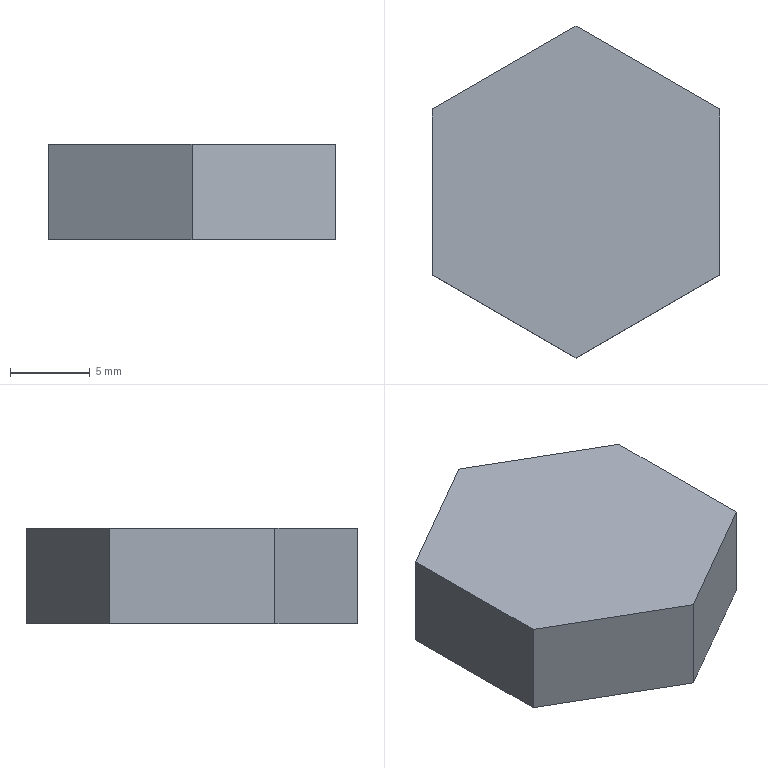Part | NX | features solid 2 | 1 solid | 8 faces | box 18 x 20.785 x 6 mm | volume 1684 mm3 | plane 8
STEP:
#1=CARTESIAN_POINT('',(-643.5,-145.196,-91.));
#2=VERTEX_POINT('',#1);
#3=CARTESIAN_POINT('',(-643.5,-134.804,-91.));
#4=VERTEX_POINT('',#3);
#5=CARTESIAN_POINT('',(-643.5,-145.196,-91.));
#6=DIRECTION('',(0.,1.,0.));
#7=VECTOR('',#6,1000.);
#8=LINE('',#5,#7);
#9=EDGE_CURVE('',#2,#4,#8,.T.);
#10=ORIENTED_EDGE('',*,*,#9,.F.);
#11=CARTESIAN_POINT('',(-643.5,-145.196,-97.));
#12=VERTEX_POINT('',#11);
#13=CARTESIAN_POINT('',(-643.5,-145.196,-97.));
#14=DIRECTION('',(0.,0.,1.));
#15=VECTOR('',#14,1000.);
#16=LINE('',#13,#15);
#17=EDGE_CURVE('',#12,#2,#16,.T.);
#18=ORIENTED_EDGE('',*,*,#17,.F.);
#19=CARTESIAN_POINT('',(-643.5,-134.804,-97.));
#20=VERTEX_POINT('',#19);
#21=CARTESIAN_POINT('',(-643.5,-145.196,-97.));
#22=DIRECTION('',(0.,1.,0.));
#23=VECTOR('',#22,1000.);
#24=LINE('',#21,#23);
#25=EDGE_CURVE('',#12,#20,#24,.T.);
#26=ORIENTED_EDGE('',*,*,#25,.T.);
#27=CARTESIAN_POINT('',(-643.5,-134.804,-97.));
#28=DIRECTION('',(0.,0.,1.));
#29=VECTOR('',#28,1000.);
#30=LINE('',#27,#29);
#31=EDGE_CURVE('',#20,#4,#30,.T.);
#32=ORIENTED_EDGE('',*,*,#31,.T.);
#33=EDGE_LOOP('',(#10,#18,#26,#32));
#34=FACE_BOUND('',#33,.T.);
#35=CARTESIAN_POINT('',(-643.5,-145.196,-97.));
#36=DIRECTION('',(1.,0.,0.));
#37=DIRECTION('',(0.,1.,0.));
#38=AXIS2_PLACEMENT_3D('',#35,#36,#37);
#39=PLANE('',#38);
#40=ADVANCED_FACE('',(#34),#39,.T.);
#41=CARTESIAN_POINT('',(-652.5,-129.608,-91.));
#42=VERTEX_POINT('',#41);
#43=CARTESIAN_POINT('',(-643.5,-134.804,-91.));
#44=DIRECTION('',(-0.866,0.5,0.));
#45=VECTOR('',#44,1000.);
#46=LINE('',#43,#45);
#47=EDGE_CURVE('',#4,#42,#46,.T.);
#48=ORIENTED_EDGE('',*,*,#47,.F.);
#49=ORIENTED_EDGE('',*,*,#31,.F.);
#50=CARTESIAN_POINT('',(-652.5,-129.608,-97.));
#51=VERTEX_POINT('',#50);
#52=CARTESIAN_POINT('',(-643.5,-134.804,-97.));
#53=DIRECTION('',(-0.866,0.5,0.));
#54=VECTOR('',#53,1000.);
#55=LINE('',#52,#54);
#56=EDGE_CURVE('',#20,#51,#55,.T.);
#57=ORIENTED_EDGE('',*,*,#56,.T.);
#58=CARTESIAN_POINT('',(-652.5,-129.608,-97.));
#59=DIRECTION('',(0.,0.,1.));
#60=VECTOR('',#59,1000.);
#61=LINE('',#58,#60);
#62=EDGE_CURVE('',#51,#42,#61,.T.);
#63=ORIENTED_EDGE('',*,*,#62,.T.);
#64=EDGE_LOOP('',(#48,#49,#57,#63));
#65=FACE_BOUND('',#64,.T.);
#66=CARTESIAN_POINT('',(-643.5,-134.804,-97.));
#67=DIRECTION('',(0.5,0.866,0.));
#68=DIRECTION('',(-0.866,0.5,0.));
#69=AXIS2_PLACEMENT_3D('',#66,#67,#68);
#70=PLANE('',#69);
#71=ADVANCED_FACE('',(#65),#70,.T.);
#72=CARTESIAN_POINT('',(-661.5,-134.804,-91.));
#73=VERTEX_POINT('',#72);
#74=CARTESIAN_POINT('',(-652.5,-129.608,-91.));
#75=DIRECTION('',(-0.866,-0.5,0.));
#76=VECTOR('',#75,1000.);
#77=LINE('',#74,#76);
#78=EDGE_CURVE('',#42,#73,#77,.T.);
#79=ORIENTED_EDGE('',*,*,#78,.F.);
#80=ORIENTED_EDGE('',*,*,#62,.F.);
#81=CARTESIAN_POINT('',(-661.5,-134.804,-97.));
#82=VERTEX_POINT('',#81);
#83=CARTESIAN_POINT('',(-652.5,-129.608,-97.));
#84=DIRECTION('',(-0.866,-0.5,0.));
#85=VECTOR('',#84,1000.);
#86=LINE('',#83,#85);
#87=EDGE_CURVE('',#51,#82,#86,.T.);
#88=ORIENTED_EDGE('',*,*,#87,.T.);
#89=CARTESIAN_POINT('',(-661.5,-134.804,-97.));
#90=DIRECTION('',(0.,0.,1.));
#91=VECTOR('',#90,1000.);
#92=LINE('',#89,#91);
#93=EDGE_CURVE('',#82,#73,#92,.T.);
#94=ORIENTED_EDGE('',*,*,#93,.T.);
#95=EDGE_LOOP('',(#79,#80,#88,#94));
#96=FACE_BOUND('',#95,.T.);
#97=CARTESIAN_POINT('',(-652.5,-129.608,-97.));
#98=DIRECTION('',(-0.5,0.866,0.));
#99=DIRECTION('',(-0.866,-0.5,0.));
#100=AXIS2_PLACEMENT_3D('',#97,#98,#99);
#101=PLANE('',#100);
#102=ADVANCED_FACE('',(#96),#101,.T.);
#103=CARTESIAN_POINT('',(-661.5,-145.196,-91.));
#104=VERTEX_POINT('',#103);
#105=CARTESIAN_POINT('',(-661.5,-134.804,-91.));
#106=DIRECTION('',(0.,-1.,0.));
#107=VECTOR('',#106,1000.);
#108=LINE('',#105,#107);
#109=EDGE_CURVE('',#73,#104,#108,.T.);
#110=ORIENTED_EDGE('',*,*,#109,.F.);
#111=ORIENTED_EDGE('',*,*,#93,.F.);
#112=CARTESIAN_POINT('',(-661.5,-145.196,-97.));
#113=VERTEX_POINT('',#112);
#114=CARTESIAN_POINT('',(-661.5,-134.804,-97.));
#115=DIRECTION('',(0.,-1.,0.));
#116=VECTOR('',#115,1000.);
#117=LINE('',#114,#116);
#118=EDGE_CURVE('',#82,#113,#117,.T.);
#119=ORIENTED_EDGE('',*,*,#118,.T.);
#120=CARTESIAN_POINT('',(-661.5,-145.196,-97.));
#121=DIRECTION('',(0.,0.,1.));
#122=VECTOR('',#121,1000.);
#123=LINE('',#120,#122);
#124=EDGE_CURVE('',#113,#104,#123,.T.);
#125=ORIENTED_EDGE('',*,*,#124,.T.);
#126=EDGE_LOOP('',(#110,#111,#119,#125));
#127=FACE_BOUND('',#126,.T.);
#128=CARTESIAN_POINT('',(-661.5,-134.804,-97.));
#129=DIRECTION('',(-1.,0.,0.));
#130=DIRECTION('',(0.,-1.,0.));
#131=AXIS2_PLACEMENT_3D('',#128,#129,#130);
#132=PLANE('',#131);
#133=ADVANCED_FACE('',(#127),#132,.T.);
#134=CARTESIAN_POINT('',(-652.5,-150.392,-91.));
#135=VERTEX_POINT('',#134);
#136=CARTESIAN_POINT('',(-661.5,-145.196,-91.));
#137=DIRECTION('',(0.866,-0.5,0.));
#138=VECTOR('',#137,1000.);
#139=LINE('',#136,#138);
#140=EDGE_CURVE('',#104,#135,#139,.T.);
#141=ORIENTED_EDGE('',*,*,#140,.F.);
#142=ORIENTED_EDGE('',*,*,#124,.F.);
#143=CARTESIAN_POINT('',(-652.5,-150.392,-97.));
#144=VERTEX_POINT('',#143);
#145=CARTESIAN_POINT('',(-661.5,-145.196,-97.));
#146=DIRECTION('',(0.866,-0.5,0.));
#147=VECTOR('',#146,1000.);
#148=LINE('',#145,#147);
#149=EDGE_CURVE('',#113,#144,#148,.T.);
#150=ORIENTED_EDGE('',*,*,#149,.T.);
#151=CARTESIAN_POINT('',(-652.5,-150.392,-97.));
#152=DIRECTION('',(0.,0.,1.));
#153=VECTOR('',#152,1000.);
#154=LINE('',#151,#153);
#155=EDGE_CURVE('',#144,#135,#154,.T.);
#156=ORIENTED_EDGE('',*,*,#155,.T.);
#157=EDGE_LOOP('',(#141,#142,#150,#156));
#158=FACE_BOUND('',#157,.T.);
#159=CARTESIAN_POINT('',(-661.5,-145.196,-97.));
#160=DIRECTION('',(-0.5,-0.866,0.));
#161=DIRECTION('',(0.866,-0.5,0.));
#162=AXIS2_PLACEMENT_3D('',#159,#160,#161);
#163=PLANE('',#162);
#164=ADVANCED_FACE('',(#158),#163,.T.);
#165=CARTESIAN_POINT('',(-652.5,-150.392,-91.));
#166=DIRECTION('',(0.866,0.5,0.));
#167=VECTOR('',#166,1000.);
#168=LINE('',#165,#167);
#169=EDGE_CURVE('',#135,#2,#168,.T.);
#170=ORIENTED_EDGE('',*,*,#169,.F.);
#171=ORIENTED_EDGE('',*,*,#155,.F.);
#172=CARTESIAN_POINT('',(-652.5,-150.392,-97.));
#173=DIRECTION('',(0.866,0.5,0.));
#174=VECTOR('',#173,1000.);
#175=LINE('',#172,#174);
#176=EDGE_CURVE('',#144,#12,#175,.T.);
#177=ORIENTED_EDGE('',*,*,#176,.T.);
#178=ORIENTED_EDGE('',*,*,#17,.T.);
#179=EDGE_LOOP('',(#170,#171,#177,#178));
#180=FACE_BOUND('',#179,.T.);
#181=CARTESIAN_POINT('',(-652.5,-150.392,-97.));
#182=DIRECTION('',(0.5,-0.866,0.));
#183=DIRECTION('',(0.866,0.5,0.));
#184=AXIS2_PLACEMENT_3D('',#181,#182,#183);
#185=PLANE('',#184);
#186=ADVANCED_FACE('',(#180),#185,.T.);
#187=ORIENTED_EDGE('',*,*,#25,.F.);
#188=ORIENTED_EDGE('',*,*,#176,.F.);
#189=ORIENTED_EDGE('',*,*,#149,.F.);
#190=ORIENTED_EDGE('',*,*,#118,.F.);
#191=ORIENTED_EDGE('',*,*,#87,.F.);
#192=ORIENTED_EDGE('',*,*,#56,.F.);
#193=EDGE_LOOP('',(#187,#188,#189,#190,#191,#192));
#194=FACE_BOUND('',#193,.T.);
#195=CARTESIAN_POINT('',(-643.5,-134.804,-97.));
#196=DIRECTION('',(0.,0.,1.));
#197=DIRECTION('',(0.,1.,0.));
#198=AXIS2_PLACEMENT_3D('',#195,#196,#197);
#199=PLANE('',#198);
#200=ADVANCED_FACE('',(#194),#199,.F.);
#201=ORIENTED_EDGE('',*,*,#9,.T.);
#202=ORIENTED_EDGE('',*,*,#47,.T.);
#203=ORIENTED_EDGE('',*,*,#78,.T.);
#204=ORIENTED_EDGE('',*,*,#109,.T.);
#205=ORIENTED_EDGE('',*,*,#140,.T.);
#206=ORIENTED_EDGE('',*,*,#169,.T.);
#207=EDGE_LOOP('',(#201,#202,#203,#204,#205,#206));
#208=FACE_BOUND('',#207,.T.);
#209=CARTESIAN_POINT('',(-643.5,-134.804,-91.));
#210=DIRECTION('',(0.,0.,1.));
#211=DIRECTION('',(0.,1.,0.));
#212=AXIS2_PLACEMENT_3D('',#209,#210,#211);
#213=PLANE('',#212);
#214=ADVANCED_FACE('',(#208),#213,.T.);
#215=CLOSED_SHELL('',(#40,#71,#102,#133,#164,#186,#200,#214));
#216=MANIFOLD_SOLID_BREP('',#215);
#217=(LENGTH_UNIT()NAMED_UNIT(*)SI_UNIT(.MILLI.,.METRE.));
#218=UNCERTAINTY_MEASURE_WITH_UNIT(LENGTH_MEASURE(0.00001),#217,'','');
#219=(NAMED_UNIT(*)PLANE_ANGLE_UNIT()SI_UNIT($,.RADIAN.));
#220=(NAMED_UNIT(*)SI_UNIT($,.STERADIAN.)SOLID_ANGLE_UNIT());
#221=(GEOMETRIC_REPRESENTATION_CONTEXT(3)GLOBAL_UNCERTAINTY_ASSIGNED_CONTEXT((#218))GLOBAL_UNIT_ASSIGNED_CONTEXT((#217,#219,#220))REPRESENTATION_CONTEXT('',''));
#222=ADVANCED_BREP_SHAPE_REPRESENTATION('',(#216),#221);